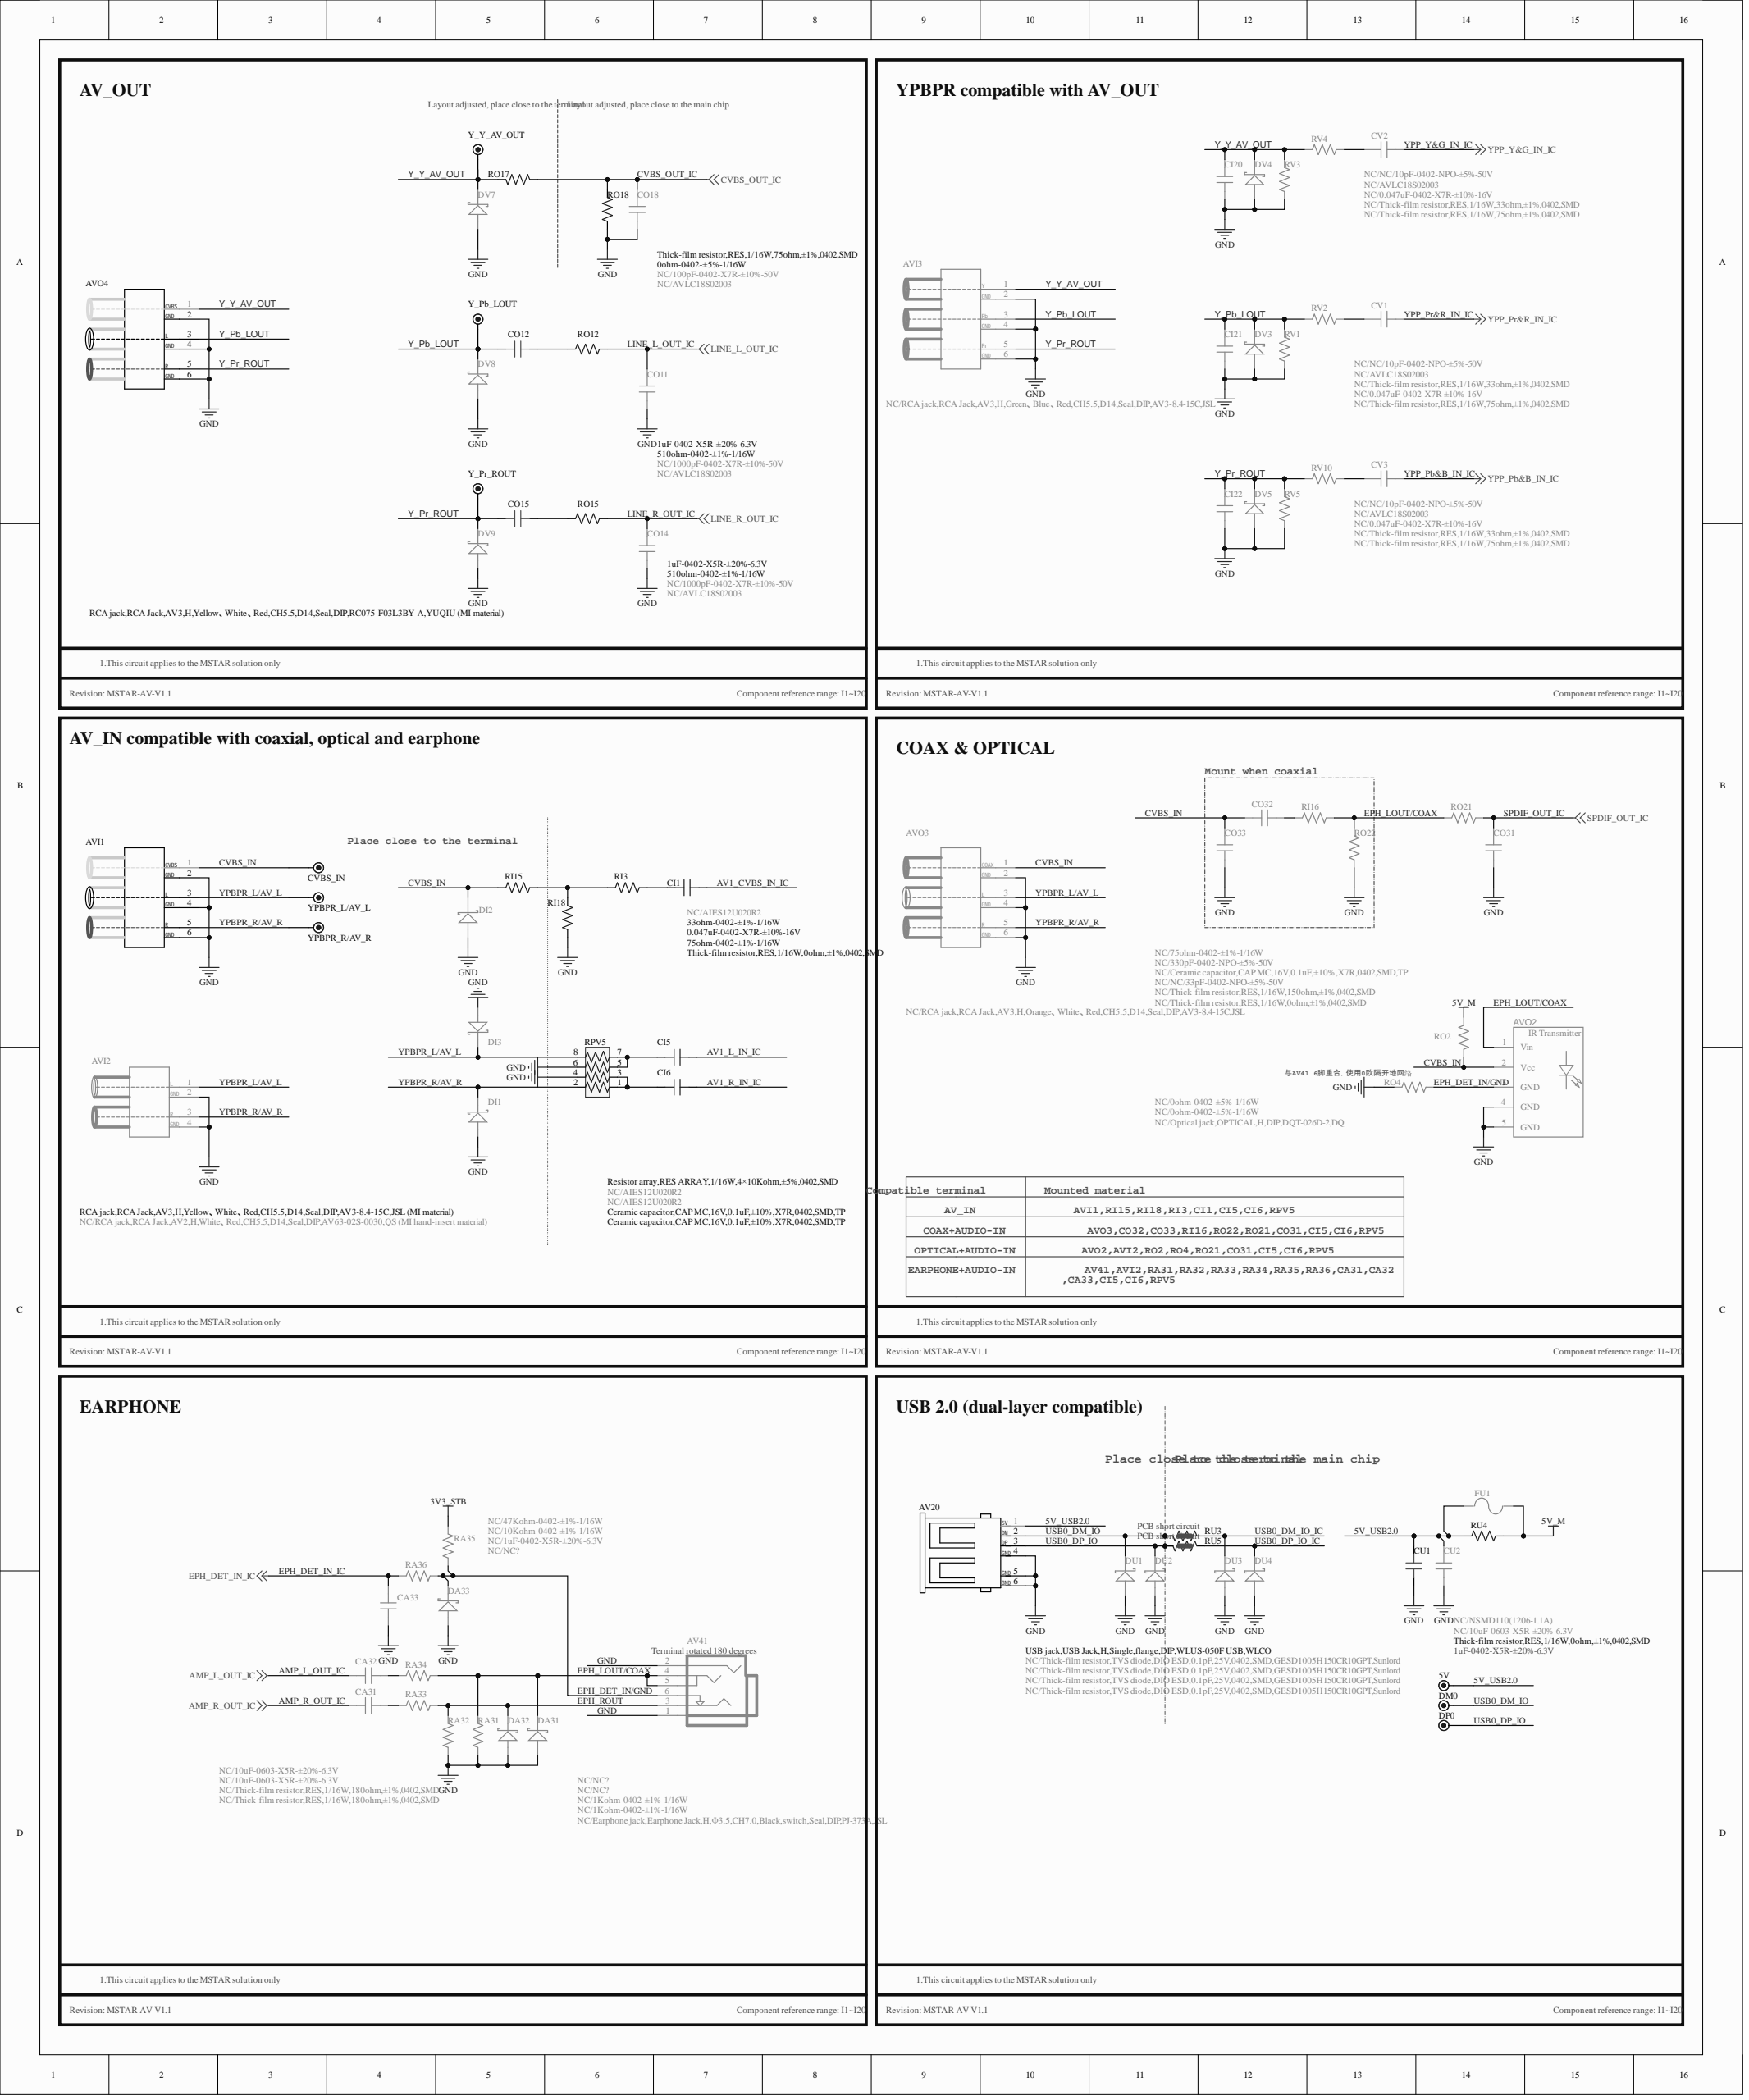Circuit board | Altium Designer | 527 parts | 243 nets | one sheet of the schematic
Parts on this sheet (reference | value | footprint):
5V | DM0 | TP
AV20 | USB jack,USB Jack,H,Single,flange,DIP,WLUS-050F USB,WLCO | USB1-HD-2
AV41 | NC/Earphone jack,Earphone Jack,H,F3.5,CH7.0,Black,switch,Seal,DIP,PJ-373A,JSL | PHONE-HD-42
AVI1 | RCA jack,RCA Jack,AV3,H,Yellow、White、Red,CH5.5,D14,Seal,DIP,AV3-8.4-15C,JSL (MI material) | AV3-H14-15
AVI2 | NC/RCA jack,RCA Jack,AV2,H,White、Red,CH5.5,D14,Seal,DIP,AV63-02S-0030,QS (MI hand-insert material) | AV2-H14-15
AVI3 | NC/RCA jack,RCA Jack,AV3,H,Green、Blue、Red,CH5.5,D14,Seal,DIP,AV3-8.4-15C,JSL | AV3-H14-15
AVO2 | NC/Optical jack,OPTICAL,H,DIP,DQT-026D-2,DQ | OPTICAL-HD-3
AVO3 | NC/RCA jack,RCA Jack,AV3,H,Orange、White、Red,CH5.5,D14,Seal,DIP,AV3-8.4-15C,JSL | AV3-H14-15
AVO4 | RCA jack,RCA Jack,AV3,H,Yellow、White、Red,CH5.5,D14,Seal,DIP,RC075-F03L3BY-A,YUQIU (MI material) | AV3-H14-15
CA31 | NC/10uF-0603-X5R-±20%-6.3V | C0603
CA32 | NC/10uF-0603-X5R-±20%-6.3V | C0603
CA33 | NC/1uF-0402-X5R-±20%-6.3V | C0402
CI1 | 0.047uF-0402-X7R-±10%-16V | C0402
CI5 | Ceramic capacitor,CAP MC,16V,0.1uF,±10%,X7R,0402,SMD,TP | C0402
CI6 | Ceramic capacitor,CAP MC,16V,0.1uF,±10%,X7R,0402,SMD,TP | C0402
CI20 | NC/NC/10pF-0402-NPO-±5%-50V | C0402
CI21 | NC/NC/10pF-0402-NPO-±5%-50V | C0402
CI22 | NC/NC/10pF-0402-NPO-±5%-50V | C0402
CO11 | NC/1000pF-0402-X7R-±10%-50V | C0402
CO12 | 1uF-0402-X5R-±20%-6.3V | C0402
CO14 | NC/1000pF-0402-X7R-±10%-50V | C0402
CO15 | 1uF-0402-X5R-±20%-6.3V | C0402
CO18 | NC/100pF-0402-X7R-±10%-50V | C0402
CO31 | NC/NC/33pF-0402-NPO-±5%-50V | C0402
CO32 | NC/Ceramic capacitor,CAP MC,16V,0.1uF,±10%,X7R,0402,SMD,TP | C0402
CO33 | NC/330pF-0402-NPO-±5%-50V | C0402
CU1 | 1uF-0402-X5R-±20%-6.3V | C0402
CU2 | NC/10uF-0603-X5R-±20%-6.3V | C0603
CV1 | NC/0.047uF-0402-X7R-±10%-16V | C0402
CV2 | NC/0.047uF-0402-X7R-±10%-16V | C0402
CV3 | NC/0.047uF-0402-X7R-±10%-16V | C0402
CVBS_IN | DM0 | TP
DA31 | NC/NC? | DIODE-S0402
DA32 | NC/NC? | DIODE-S0402
DA33 | NC/NC? | DIODE-S0402
DI1 | NC/AIES12U020R2 | DIODE-S0402
DI2 | NC/AIES12U020R2 | DIODE-S0402
DI3 | NC/AIES12U020R2 | DIODE-S0402
DM0 | DM0 | TP
DP0 | DM0 | TP
DU1 | NC/Thick-film resistor,TVS diode,DIO ESD,0.1pF,25V,0402,SMD,GESD1005H150CR10GPT,Sunlord | DIODE-S0402
DU2 | NC/Thick-film resistor,TVS diode,DIO ESD,0.1pF,25V,0402,SMD,GESD1005H150CR10GPT,Sunlord | DIODE-S0402
DU3 | NC/Thick-film resistor,TVS diode,DIO ESD,0.1pF,25V,0402,SMD,GESD1005H150CR10GPT,Sunlord | DIODE-S0402
DU4 | NC/Thick-film resistor,TVS diode,DIO ESD,0.1pF,25V,0402,SMD,GESD1005H150CR10GPT,Sunlord | DIODE-S0402
DV3 | NC/AVLC18S02003 | DIODE-S0402
DV4 | NC/AVLC18S02003 | DIODE-S0402
DV5 | NC/AVLC18S02003 | DIODE-S0402
DV7 | NC/AVLC18S02003 | DIODE-S0402
DV8 | NC/AVLC18S02003 | DIODE-S0402
DV9 | NC/AVLC18S02003 | DIODE-S0402
FU1 | NC/NSMD110(1206-1.1A) | FUSE1.1A-S
RA31 | NC/1Kohm-0402-±1%-1/16W | R0402
RA32 | NC/1Kohm-0402-±1%-1/16W | R0402
RA33 | NC/Thick-film resistor,RES,1/16W,180ohm,±1%,0402,SMD | R0402
RA34 | NC/Thick-film resistor,RES,1/16W,180ohm,±1%,0402,SMD | R0402
RA35 | NC/47Kohm-0402-±1%-1/16W | R0402
RA36 | NC/10Kohm-0402-±1%-1/16W | R0402
RI3 | 33ohm-0402-±1%-1/16W | R0402
RI15 | Thick-film resistor,RES,1/16W,0ohm,±1%,0402,SMD | R0402
RI16 | NC/Thick-film resistor,RES,1/16W,0ohm,±1%,0402,SMD | R0402
RI18 | 75ohm-0402-±1%-1/16W | R0402
RO2 | NC/0ohm-0402-±5%-1/16W | R0402
RO4 | NC/0ohm-0402-±5%-1/16W | R0402
RO12 | 510ohm-0402-±1%-1/16W | R0402
RO15 | 510ohm-0402-±1%-1/16W | R0402
RO17 | 0ohm-0402-±5%-1/16W | R0402
RO18 | Thick-film resistor,RES,1/16W,75ohm,±1%,0402,SMD | R0402
RO21 | NC/Thick-film resistor,RES,1/16W,150ohm,±1%,0402,SMD | R0402
RO22 | NC/75ohm-0402-±1%-1/16W | R0402
RPV5 | Resistor array,RES ARRAY,1/16W,4×10Kohm,±5%,0402,SMD | RA0402
RU3 | NC/0ohm-0402-PCB | R0402SC
RU4 | Thick-film resistor,RES,1/16W,0ohm,±1%,0402,SMD | R0402
RU5 | NC/0ohm-0402-PCB | R0402SC
RV1 | NC/Thick-film resistor,RES,1/16W,75ohm,±1%,0402,SMD | R0402
RV2 | NC/Thick-film resistor,RES,1/16W,33ohm,±1%,0402,SMD | R0402
RV3 | NC/Thick-film resistor,RES,1/16W,75ohm,±1%,0402,SMD | R0402
RV4 | NC/Thick-film resistor,RES,1/16W,33ohm,±1%,0402,SMD | R0402
RV5 | NC/Thick-film resistor,RES,1/16W,75ohm,±1%,0402,SMD | R0402
RV10 | NC/Thick-film resistor,RES,1/16W,33ohm,±1%,0402,SMD | R0402
Y_Pb_LOUT | DM0 | TP
Y_Pr_ROUT | DM0 | TP
Y_Y_AV_OUT | DM0 | TP
YPBPR_L/AV_L | DM0 | TP
YPBPR_R/AV_R | DM0 | TP
Nets of these parts (net: part-pin ...):
YPP_Y&G_IN_IC: CV2-2
YPP_Pr&R_IN_IC: CV1-2
YPP_Pb&B_IN_IC: CV3-2
YPBPR_R/AV_R: AVI1-5 AVI2-3 AVO3-5 DI1-K RPV5-2 YPBPR_R/AV_R-1
YPBPR_L/AV_L: AVI1-3 AVI2-1 AVO3-3 DI3-K RPV5-8 YPBPR_L/AV_L-1
Y_Y_AV_OUT: AVI3-1 AVO4-1 CI20-1 DV4-K DV7-K RO17-2 RV3-2 RV4-1 Y_Y_AV_OUT-1
Y_Pr_ROUT: AVI3-5 AVO4-5 CI22-1 CO15-2 DV5-K DV9-K RV5-2 RV10-1 Y_Pr_ROUT-1
Y_Pb_LOUT: AVI3-3 AVO4-3 CI21-1 CO12-2 DV3-K DV8-K RV1-2 RV2-1 Y_Pb_LOUT-1
USB0_DP_IO_IC: DU4-K RU5-1
USB0_DP_IO: AV20-3 DP0-1 DU2-K RU5-2 RU5-3
USB0_DM_IO_IC: DU3-K RU3-1
USB0_DM_IO: AV20-2 DM0-1 DU1-K RU3-2 RU3-3
SPDIF_OUT_IC: CO31-2 RO21-2
NetRI3_1: RI3-1 RI15-2 RI18-2
NetCV3_1: CV3-1 RV10-2
NetCV2_1: CV2-1 RV4-2
NetCV1_1: CV1-1 RV2-2
NetCO32_1: CO32-1 RI16-1
NetCO15_1: CO15-1 RO15-2
NetCO12_1: CO12-1 RO12-2
NetCI6_2: CI6-2 RPV5-1 RPV5-3
NetCI5_2: CI5-2 RPV5-5 RPV5-7
NetCI1_2: CI1-2 RI3-2
NetCA32_1: CA32-1 RA34-1
NetCA31_1: CA31-1 RA33-1
LINE_R_OUT_IC: CO14-2 RO15-1
LINE_L_OUT_IC: CO11-2 RO12-1
GND: AV20-4 AV20-5 AV20-6 AV41-1 AV41-2 AVI1-2 AVI1-4 AVI1-6 AVI2-2 AVI2-4 AVI3-2 AVI3-4 AVI3-6 AVO2-4 AVO2-5 AVO3-2 AVO3-4 AVO3-6 AVO4-2 AVO4-4 AVO4-6 CA33-1 CI20-2 CI21-2 CI22-2 CO11-1 CO14-1 CO18-1 CO31-1 CO33-1 CU1-2 CU2-2 DA31-A DA32-A DA33-A DI1-A DI2-A DI3-A DU1-A DU2-A DU3-A DU4-A DV3-A DV4-A DV5-A DV7-A DV8-A DV9-A RA31-1 RA32-1 RI18-1 RO4-1 RO18-1 RO22-1 RPV5-4 RPV5-6 RV1-1 RV3-1 RV5-1
EPH_ROUT: AV41-3 DA32-K RA32-2 RA33-2
EPH_LOUT/COAX: AV41-4 AV41-5 AVO2-1 DA31-K RA31-2 RA34-2 RI16-2 RO21-1 RO22-2
EPH_DET_IN_IC: CA33-2 RA36-1
EPH_DET_IN/GND: AV41-6 AVO2-3 DA33-K RA35-1 RA36-2 RO4-2
CVBS_OUT_IC: CO18-2 RO17-1 RO18-2
CVBS_IN: AVI1-1 AVO2-2 AVO3-1 CO32-2 CO33-2 CVBS_IN-1 DI2-K RI15-1 RO2-2
AV1_R_IN_IC: CI6-1
AV1_L_IN_IC: CI5-1
AV1_CVBS_IN_IC: CI1-1
AMP_R_OUT_IC: CA31-2
AMP_L_OUT_IC: CA32-2
5V_USB2.0: 5V-1 AV20-1 CU1-1 CU2-1 FU1-1 RU4-1
5V_M: FU1-2 RO2-1 RU4-2
3V3_STB: RA35-2